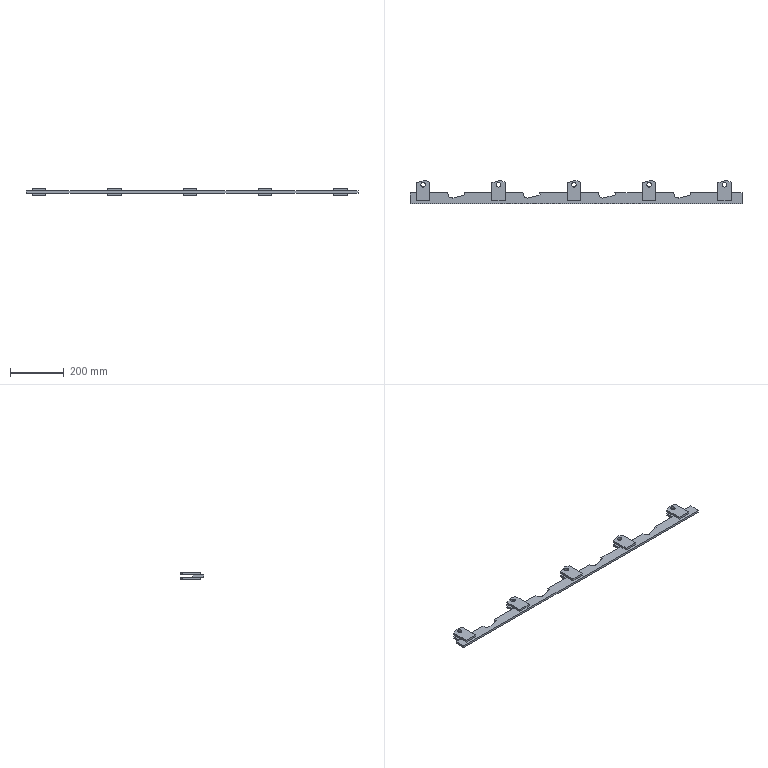Part | STEP file | Bar screen plate 4_Default<As machined> | 11 solids | 116 faces | box 1234 x 86.845 x 24 mm | volume 638578 mm3 | plane 92 | cylinder 24 | commonest cylinder face diameters 17 x20 30 x4